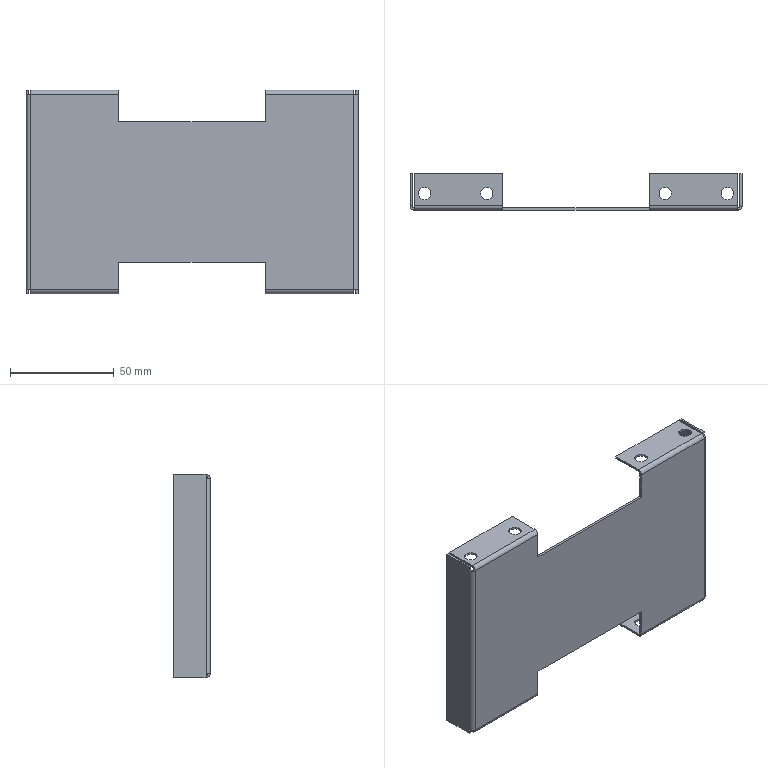Part | SolidWorks | features BaseBody 1 | 1 solid | 70 faces | box 160 x 17.5 x 98 mm | volume 19104 mm3 | plane 42 | cylinder 28 | commonest cylinder face diameters 6 x16 2 x6 4 x6